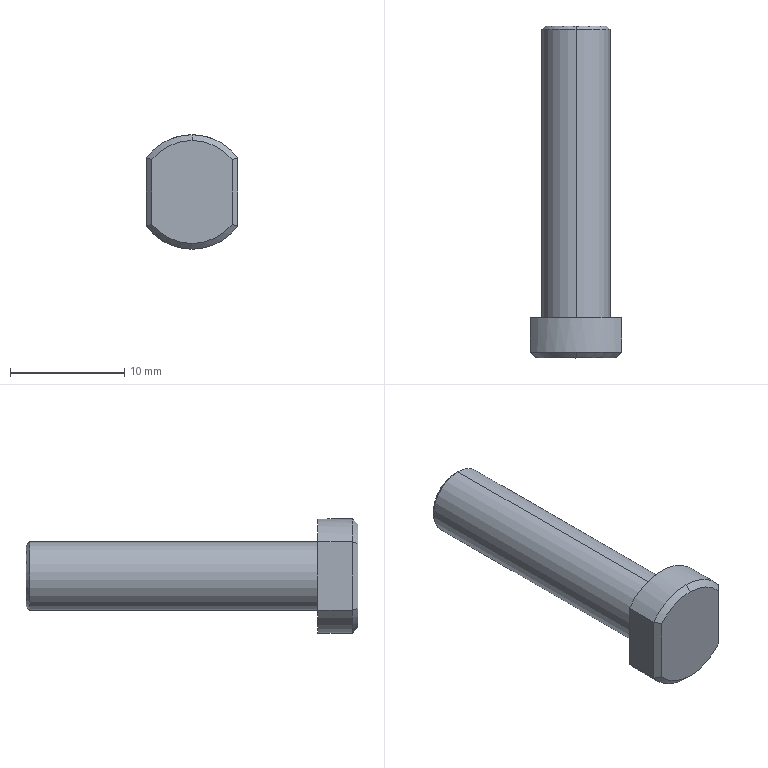Part | SolidWorks | features BaseBody 1 | 1 solid | 21 faces | box 8 x 29 x 10 mm | volume 861.581 mm3 | cone 7 | cylinder 7 | plane 7 | commonest cylinder face diameters 10 x3 3.3 x2 6 x2
STEP:
#1=CARTESIAN_POINT('',(0.,29.,2.7));
#2=VERTEX_POINT('',#1);
#3=CARTESIAN_POINT('',(0.,28.7,3.));
#4=VERTEX_POINT('',#3);
#5=CARTESIAN_POINT('',(0.,29.,2.7));
#6=DIRECTION('',(0.,-0.7071,0.7071));
#7=VECTOR('',#6,1000.);
#8=LINE('',#5,#7);
#9=EDGE_CURVE('',#2,#4,#8,.T.);
#10=ORIENTED_EDGE('',*,*,#9,.F.);
#11=CARTESIAN_POINT('',(0.,29.,-2.7));
#12=VERTEX_POINT('',#11);
#13=CARTESIAN_POINT('',(0.,29.,0.));
#14=DIRECTION('',(0.,1.,0.));
#15=DIRECTION('',(0.,0.,1.));
#16=AXIS2_PLACEMENT_3D('',#13,#14,#15);
#17=CIRCLE('',#16,2.7);
#18=EDGE_CURVE('',#12,#2,#17,.T.);
#19=ORIENTED_EDGE('',*,*,#18,.F.);
#20=CARTESIAN_POINT('',(0.,28.7,-3.));
#21=VERTEX_POINT('',#20);
#22=CARTESIAN_POINT('',(0.,29.,-2.7));
#23=DIRECTION('',(0.,-0.7071,-0.7071));
#24=VECTOR('',#23,1000.);
#25=LINE('',#22,#24);
#26=EDGE_CURVE('',#12,#21,#25,.T.);
#27=ORIENTED_EDGE('',*,*,#26,.T.);
#28=CARTESIAN_POINT('',(0.,28.7,0.));
#29=DIRECTION('',(0.,-1.,0.));
#30=DIRECTION('',(0.,0.,1.));
#31=AXIS2_PLACEMENT_3D('',#28,#29,#30);
#32=CIRCLE('',#31,3.);
#33=EDGE_CURVE('',#4,#21,#32,.T.);
#34=ORIENTED_EDGE('',*,*,#33,.F.);
#35=EDGE_LOOP('',(#10,#19,#27,#34));
#36=FACE_OUTER_BOUND('',#35,.T.);
#37=CARTESIAN_POINT('',(0.,29.,0.));
#38=DIRECTION('',(0.,-1.,0.));
#39=DIRECTION('',(0.,0.,-1.));
#40=AXIS2_PLACEMENT_3D('',#37,#38,#39);
#41=CONICAL_SURFACE('',#40,2.7,0.7854);
#42=ADVANCED_FACE('',(#36),#41,.T.);
#43=CARTESIAN_POINT('',(0.,17.5,-1.65));
#44=VERTEX_POINT('',#43);
#45=CARTESIAN_POINT('',(0.,29.,-1.65));
#46=VERTEX_POINT('',#45);
#47=CARTESIAN_POINT('',(0.,29.,-1.65));
#48=DIRECTION('',(0.,1.,0.));
#49=VECTOR('',#48,1000.);
#50=LINE('',#47,#49);
#51=EDGE_CURVE('',#44,#46,#50,.T.);
#52=ORIENTED_EDGE('',*,*,#51,.F.);
#53=CARTESIAN_POINT('',(0.,17.5,1.65));
#54=VERTEX_POINT('',#53);
#55=CARTESIAN_POINT('',(0.,17.5,0.));
#56=DIRECTION('',(0.,1.,0.));
#57=DIRECTION('',(0.,0.,1.));
#58=AXIS2_PLACEMENT_3D('',#55,#56,#57);
#59=CIRCLE('',#58,1.65);
#60=EDGE_CURVE('',#54,#44,#59,.T.);
#61=ORIENTED_EDGE('',*,*,#60,.F.);
#62=CARTESIAN_POINT('',(0.,29.,1.65));
#63=VERTEX_POINT('',#62);
#64=CARTESIAN_POINT('',(0.,29.,1.65));
#65=DIRECTION('',(0.,1.,0.));
#66=VECTOR('',#65,1000.);
#67=LINE('',#64,#66);
#68=EDGE_CURVE('',#54,#63,#67,.T.);
#69=ORIENTED_EDGE('',*,*,#68,.T.);
#70=CARTESIAN_POINT('',(0.,29.,0.));
#71=DIRECTION('',(0.,1.,0.));
#72=DIRECTION('',(0.,0.,1.));
#73=AXIS2_PLACEMENT_3D('',#70,#71,#72);
#74=CIRCLE('',#73,1.65);
#75=EDGE_CURVE('',#63,#46,#74,.T.);
#76=ORIENTED_EDGE('',*,*,#75,.T.);
#77=EDGE_LOOP('',(#52,#61,#69,#76));
#78=FACE_OUTER_BOUND('',#77,.T.);
#79=CARTESIAN_POINT('',(0.,29.,0.));
#80=DIRECTION('',(0.,1.,0.));
#81=DIRECTION('',(0.,0.,1.));
#82=AXIS2_PLACEMENT_3D('',#79,#80,#81);
#83=CYLINDRICAL_SURFACE('',#82,1.65);
#84=ADVANCED_FACE('',(#78),#83,.F.);
#85=CARTESIAN_POINT('',(0.,16.509,0.));
#86=VERTEX_POINT('',#85);
#87=CARTESIAN_POINT('',(0.,17.5,-1.65));
#88=DIRECTION('',(0.,0.515,-0.8572));
#89=VECTOR('',#88,1000.);
#90=LINE('',#87,#89);
#91=EDGE_CURVE('',#86,#44,#90,.T.);
#92=ORIENTED_EDGE('',*,*,#91,.F.);
#93=CARTESIAN_POINT('',(0.,17.5,1.65));
#94=DIRECTION('',(0.,0.515,0.8572));
#95=VECTOR('',#94,1000.);
#96=LINE('',#93,#95);
#97=EDGE_CURVE('',#86,#54,#96,.T.);
#98=ORIENTED_EDGE('',*,*,#97,.T.);
#99=ORIENTED_EDGE('',*,*,#60,.T.);
#100=EDGE_LOOP('',(#92,#98,#99));
#101=FACE_OUTER_BOUND('',#100,.T.);
#102=CARTESIAN_POINT('',(0.,17.5,0.));
#103=DIRECTION('',(0.,1.,0.));
#104=DIRECTION('',(0.,0.,1.));
#105=AXIS2_PLACEMENT_3D('',#102,#103,#104);
#106=CONICAL_SURFACE('',#105,1.65,1.03);
#107=ADVANCED_FACE('',(#101),#106,.F.);
#108=CARTESIAN_POINT('',(4.,0.5,3.));
#109=VERTEX_POINT('',#108);
#110=CARTESIAN_POINT('',(3.5,0.,2.828));
#111=VERTEX_POINT('',#110);
#112=CARTESIAN_POINT('',(4.,0.5,3.));
#113=CARTESIAN_POINT('',(3.833,0.3331,2.944));
#114=CARTESIAN_POINT('',(3.666,0.1664,2.887));
#115=CARTESIAN_POINT('',(3.5,0.,2.828));
#116=B_SPLINE_CURVE_WITH_KNOTS('',3,(#112,#113,#114,#115),.UNSPECIFIED.,.F.,.F.,(4,4),(0.,0.0007276),.UNSPECIFIED.);
#117=EDGE_CURVE('',#109,#111,#116,.T.);
#118=ORIENTED_EDGE('',*,*,#117,.T.);
#119=CARTESIAN_POINT('',(3.5,0.,-2.828));
#120=VERTEX_POINT('',#119);
#121=CARTESIAN_POINT('',(3.5,0.,0.));
#122=DIRECTION('',(0.,0.,1.));
#123=VECTOR('',#122,1000.);
#124=LINE('',#121,#123);
#125=EDGE_CURVE('',#120,#111,#124,.T.);
#126=ORIENTED_EDGE('',*,*,#125,.F.);
#127=CARTESIAN_POINT('',(4.,0.5,-3.));
#128=VERTEX_POINT('',#127);
#129=CARTESIAN_POINT('',(3.5,0.,-2.828));
#130=CARTESIAN_POINT('',(3.666,0.1664,-2.887));
#131=CARTESIAN_POINT('',(3.833,0.3331,-2.944));
#132=CARTESIAN_POINT('',(4.,0.5,-3.));
#133=B_SPLINE_CURVE_WITH_KNOTS('',3,(#129,#130,#131,#132),.UNSPECIFIED.,.F.,.F.,(4,4),(0.,0.0007276),.UNSPECIFIED.);
#134=EDGE_CURVE('',#120,#128,#133,.T.);
#135=ORIENTED_EDGE('',*,*,#134,.T.);
#136=CARTESIAN_POINT('',(4.,0.5,3.));
#137=DIRECTION('',(0.,0.,-1.));
#138=VECTOR('',#137,1000.);
#139=LINE('',#136,#138);
#140=EDGE_CURVE('',#109,#128,#139,.T.);
#141=ORIENTED_EDGE('',*,*,#140,.F.);
#142=EDGE_LOOP('',(#118,#126,#135,#141));
#143=FACE_OUTER_BOUND('',#142,.T.);
#144=CARTESIAN_POINT('',(4.,0.5,3.));
#145=DIRECTION('',(-0.7071,0.7071,0.));
#146=DIRECTION('',(0.,0.,1.));
#147=AXIS2_PLACEMENT_3D('',#144,#145,#146);
#148=PLANE('',#147);
#149=ADVANCED_FACE('',(#143),#148,.F.);
#150=CARTESIAN_POINT('',(-3.5,0.,-2.828));
#151=VERTEX_POINT('',#150);
#152=CARTESIAN_POINT('',(-4.,0.5,-3.));
#153=VERTEX_POINT('',#152);
#154=CARTESIAN_POINT('',(-3.5,0.,-2.828));
#155=CARTESIAN_POINT('',(-3.666,0.1664,-2.887));
#156=CARTESIAN_POINT('',(-3.833,0.3331,-2.944));
#157=CARTESIAN_POINT('',(-4.,0.5,-3.));
#158=B_SPLINE_CURVE_WITH_KNOTS('',3,(#154,#155,#156,#157),.UNSPECIFIED.,.F.,.F.,(4,4),(0.,0.0007276),.UNSPECIFIED.);
#159=EDGE_CURVE('',#151,#153,#158,.T.);
#160=ORIENTED_EDGE('',*,*,#159,.T.);
#161=CARTESIAN_POINT('',(0.,0.5,-5.));
#162=VERTEX_POINT('',#161);
#163=CARTESIAN_POINT('',(0.,0.5,0.));
#164=DIRECTION('',(0.,1.,0.));
#165=DIRECTION('',(0.,0.,1.));
#166=AXIS2_PLACEMENT_3D('',#163,#164,#165);
#167=CIRCLE('',#166,5.);
#168=EDGE_CURVE('',#162,#153,#167,.T.);
#169=ORIENTED_EDGE('',*,*,#168,.F.);
#170=CARTESIAN_POINT('',(0.,0.5,0.));
#171=DIRECTION('',(0.,1.,0.));
#172=DIRECTION('',(0.,0.,1.));
#173=AXIS2_PLACEMENT_3D('',#170,#171,#172);
#174=CIRCLE('',#173,5.);
#175=EDGE_CURVE('',#128,#162,#174,.T.);
#176=ORIENTED_EDGE('',*,*,#175,.F.);
#177=ORIENTED_EDGE('',*,*,#134,.F.);
#178=CARTESIAN_POINT('',(0.,0.,0.));
#179=DIRECTION('',(0.,-1.,0.));
#180=DIRECTION('',(0.,0.,1.));
#181=AXIS2_PLACEMENT_3D('',#178,#179,#180);
#182=CIRCLE('',#181,4.5);
#183=EDGE_CURVE('',#151,#120,#182,.T.);
#184=ORIENTED_EDGE('',*,*,#183,.F.);
#185=EDGE_LOOP('',(#160,#169,#176,#177,#184));
#186=FACE_OUTER_BOUND('',#185,.T.);
#187=CARTESIAN_POINT('',(0.,0.5,0.));
#188=DIRECTION('',(0.,1.,0.));
#189=DIRECTION('',(0.,0.,1.));
#190=AXIS2_PLACEMENT_3D('',#187,#188,#189);
#191=CONICAL_SURFACE('',#190,5.,0.7854);
#192=ADVANCED_FACE('',(#186),#191,.T.);
#193=CARTESIAN_POINT('',(0.,0.,4.5));
#194=VERTEX_POINT('',#193);
#195=CARTESIAN_POINT('',(0.,0.5,5.));
#196=VERTEX_POINT('',#195);
#197=CARTESIAN_POINT('',(0.,0.5,5.));
#198=DIRECTION('',(0.,0.7071,0.7071));
#199=VECTOR('',#198,1000.);
#200=LINE('',#197,#199);
#201=EDGE_CURVE('',#194,#196,#200,.T.);
#202=ORIENTED_EDGE('',*,*,#201,.F.);
#203=CARTESIAN_POINT('',(0.,0.,0.));
#204=DIRECTION('',(0.,-1.,0.));
#205=DIRECTION('',(0.,0.,1.));
#206=AXIS2_PLACEMENT_3D('',#203,#204,#205);
#207=CIRCLE('',#206,4.5);
#208=EDGE_CURVE('',#111,#194,#207,.T.);
#209=ORIENTED_EDGE('',*,*,#208,.F.);
#210=ORIENTED_EDGE('',*,*,#117,.F.);
#211=CARTESIAN_POINT('',(0.,0.5,0.));
#212=DIRECTION('',(0.,1.,0.));
#213=DIRECTION('',(0.,0.,1.));
#214=AXIS2_PLACEMENT_3D('',#211,#212,#213);
#215=CIRCLE('',#214,5.);
#216=EDGE_CURVE('',#196,#109,#215,.T.);
#217=ORIENTED_EDGE('',*,*,#216,.F.);
#218=EDGE_LOOP('',(#202,#209,#210,#217));
#219=FACE_OUTER_BOUND('',#218,.T.);
#220=CARTESIAN_POINT('',(0.,0.5,0.));
#221=DIRECTION('',(0.,1.,0.));
#222=DIRECTION('',(0.,0.,1.));
#223=AXIS2_PLACEMENT_3D('',#220,#221,#222);
#224=CONICAL_SURFACE('',#223,5.,0.7854);
#225=ADVANCED_FACE('',(#219),#224,.T.);
#226=ORIENTED_EDGE('',*,*,#159,.F.);
#227=CARTESIAN_POINT('',(-3.5,0.,2.828));
#228=VERTEX_POINT('',#227);
#229=CARTESIAN_POINT('',(-3.5,0.,0.));
#230=DIRECTION('',(0.,0.,-1.));
#231=VECTOR('',#230,1000.);
#232=LINE('',#229,#231);
#233=EDGE_CURVE('',#228,#151,#232,.T.);
#234=ORIENTED_EDGE('',*,*,#233,.F.);
#235=CARTESIAN_POINT('',(-4.,0.5,3.));
#236=VERTEX_POINT('',#235);
#237=CARTESIAN_POINT('',(-4.,0.5,3.));
#238=CARTESIAN_POINT('',(-3.833,0.3331,2.944));
#239=CARTESIAN_POINT('',(-3.666,0.1664,2.887));
#240=CARTESIAN_POINT('',(-3.5,0.,2.828));
#241=B_SPLINE_CURVE_WITH_KNOTS('',3,(#237,#238,#239,#240),.UNSPECIFIED.,.F.,.F.,(4,4),(0.,0.0007276),.UNSPECIFIED.);
#242=EDGE_CURVE('',#236,#228,#241,.T.);
#243=ORIENTED_EDGE('',*,*,#242,.F.);
#244=CARTESIAN_POINT('',(-4.,0.5,3.));
#245=DIRECTION('',(0.,0.,1.));
#246=VECTOR('',#245,1000.);
#247=LINE('',#244,#246);
#248=EDGE_CURVE('',#153,#236,#247,.T.);
#249=ORIENTED_EDGE('',*,*,#248,.F.);
#250=EDGE_LOOP('',(#226,#234,#243,#249));
#251=FACE_OUTER_BOUND('',#250,.T.);
#252=CARTESIAN_POINT('',(-4.,0.5,3.));
#253=DIRECTION('',(0.7071,0.7071,0.));
#254=DIRECTION('',(0.,0.,-1.));
#255=AXIS2_PLACEMENT_3D('',#252,#253,#254);
#256=PLANE('',#255);
#257=ADVANCED_FACE('',(#251),#256,.F.);
#258=CARTESIAN_POINT('',(-4.,3.5,-3.));
#259=VERTEX_POINT('',#258);
#260=CARTESIAN_POINT('',(-4.,29.001,-3.));
#261=DIRECTION('',(0.,-1.,0.));
#262=VECTOR('',#261,1000.);
#263=LINE('',#260,#262);
#264=EDGE_CURVE('',#259,#153,#263,.T.);
#265=ORIENTED_EDGE('',*,*,#264,.T.);
#266=ORIENTED_EDGE('',*,*,#248,.T.);
#267=CARTESIAN_POINT('',(-4.,3.5,3.));
#268=VERTEX_POINT('',#267);
#269=CARTESIAN_POINT('',(-4.,29.001,3.));
#270=DIRECTION('',(0.,-1.,0.));
#271=VECTOR('',#270,1000.);
#272=LINE('',#269,#271);
#273=EDGE_CURVE('',#268,#236,#272,.T.);
#274=ORIENTED_EDGE('',*,*,#273,.F.);
#275=CARTESIAN_POINT('',(-4.,3.5,3.));
#276=DIRECTION('',(0.,0.,1.));
#277=VECTOR('',#276,1000.);
#278=LINE('',#275,#277);
#279=EDGE_CURVE('',#259,#268,#278,.T.);
#280=ORIENTED_EDGE('',*,*,#279,.F.);
#281=EDGE_LOOP('',(#265,#266,#274,#280));
#282=FACE_OUTER_BOUND('',#281,.T.);
#283=CARTESIAN_POINT('',(-4.,29.001,3.));
#284=DIRECTION('',(1.,0.,0.));
#285=DIRECTION('',(0.,1.,0.));
#286=AXIS2_PLACEMENT_3D('',#283,#284,#285);
#287=PLANE('',#286);
#288=ADVANCED_FACE('',(#282),#287,.F.);
#289=CARTESIAN_POINT('',(4.,3.5,3.));
#290=VERTEX_POINT('',#289);
#291=CARTESIAN_POINT('',(4.,29.001,3.));
#292=DIRECTION('',(0.,-1.,0.));
#293=VECTOR('',#292,1000.);
#294=LINE('',#291,#293);
#295=EDGE_CURVE('',#290,#109,#294,.T.);
#296=ORIENTED_EDGE('',*,*,#295,.T.);
#297=ORIENTED_EDGE('',*,*,#140,.T.);
#298=CARTESIAN_POINT('',(4.,3.5,-3.));
#299=VERTEX_POINT('',#298);
#300=CARTESIAN_POINT('',(4.,29.001,-3.));
#301=DIRECTION('',(0.,-1.,0.));
#302=VECTOR('',#301,1000.);
#303=LINE('',#300,#302);
#304=EDGE_CURVE('',#299,#128,#303,.T.);
#305=ORIENTED_EDGE('',*,*,#304,.F.);
#306=CARTESIAN_POINT('',(4.,3.5,3.));
#307=DIRECTION('',(0.,0.,-1.));
#308=VECTOR('',#307,1000.);
#309=LINE('',#306,#308);
#310=EDGE_CURVE('',#290,#299,#309,.T.);
#311=ORIENTED_EDGE('',*,*,#310,.F.);
#312=EDGE_LOOP('',(#296,#297,#305,#311));
#313=FACE_OUTER_BOUND('',#312,.T.);
#314=CARTESIAN_POINT('',(4.,29.001,3.));
#315=DIRECTION('',(-1.,0.,0.));
#316=DIRECTION('',(0.,0.,1.));
#317=AXIS2_PLACEMENT_3D('',#314,#315,#316);
#318=PLANE('',#317);
#319=ADVANCED_FACE('',(#313),#318,.F.);
#320=ORIENTED_EDGE('',*,*,#75,.F.);
#321=CARTESIAN_POINT('',(0.,29.,0.));
#322=DIRECTION('',(0.,1.,0.));
#323=DIRECTION('',(0.,0.,1.));
#324=AXIS2_PLACEMENT_3D('',#321,#322,#323);
#325=CIRCLE('',#324,1.65);
#326=EDGE_CURVE('',#46,#63,#325,.T.);
#327=ORIENTED_EDGE('',*,*,#326,.F.);
#328=EDGE_LOOP('',(#320,#327));
#329=FACE_BOUND('',#328,.T.);
#330=ORIENTED_EDGE('',*,*,#18,.T.);
#331=CARTESIAN_POINT('',(0.,29.,0.));
#332=DIRECTION('',(0.,1.,0.));
#333=DIRECTION('',(0.,0.,1.));
#334=AXIS2_PLACEMENT_3D('',#331,#332,#333);
#335=CIRCLE('',#334,2.7);
#336=EDGE_CURVE('',#2,#12,#335,.T.);
#337=ORIENTED_EDGE('',*,*,#336,.T.);
#338=EDGE_LOOP('',(#330,#337));
#339=FACE_OUTER_BOUND('',#338,.T.);
#340=CARTESIAN_POINT('',(0.,29.,0.));
#341=DIRECTION('',(0.,1.,0.));
#342=DIRECTION('',(1.,0.,0.));
#343=AXIS2_PLACEMENT_3D('',#340,#341,#342);
#344=PLANE('',#343);
#345=ADVANCED_FACE('',(#329,#339),#344,.T.);
#346=CARTESIAN_POINT('',(0.,3.5,-3.));
#347=VERTEX_POINT('',#346);
#348=CARTESIAN_POINT('',(0.,3.5,-3.));
#349=DIRECTION('',(0.,1.,0.));
#350=VECTOR('',#349,1000.);
#351=LINE('',#348,#350);
#352=EDGE_CURVE('',#347,#21,#351,.T.);
#353=ORIENTED_EDGE('',*,*,#352,.F.);
#354=CARTESIAN_POINT('',(0.,3.5,3.));
#355=VERTEX_POINT('',#354);
#356=CARTESIAN_POINT('',(0.,3.5,0.));
#357=DIRECTION('',(0.,1.,0.));
#358=DIRECTION('',(0.,0.,1.));
#359=AXIS2_PLACEMENT_3D('',#356,#357,#358);
#360=CIRCLE('',#359,3.);
#361=EDGE_CURVE('',#347,#355,#360,.T.);
#362=ORIENTED_EDGE('',*,*,#361,.T.);
#363=CARTESIAN_POINT('',(0.,3.5,3.));
#364=DIRECTION('',(0.,1.,0.));
#365=VECTOR('',#364,1000.);
#366=LINE('',#363,#365);
#367=EDGE_CURVE('',#355,#4,#366,.T.);
#368=ORIENTED_EDGE('',*,*,#367,.T.);
#369=ORIENTED_EDGE('',*,*,#33,.T.);
#370=EDGE_LOOP('',(#353,#362,#368,#369));
#371=FACE_OUTER_BOUND('',#370,.T.);
#372=CARTESIAN_POINT('',(0.,3.5,0.));
#373=DIRECTION('',(0.,1.,0.));
#374=DIRECTION('',(0.,0.,1.));
#375=AXIS2_PLACEMENT_3D('',#372,#373,#374);
#376=CYLINDRICAL_SURFACE('',#375,3.);
#377=ADVANCED_FACE('',(#371),#376,.T.);
#378=CARTESIAN_POINT('',(0.,3.5,0.));
#379=DIRECTION('',(0.,1.,0.));
#380=DIRECTION('',(0.,0.,1.));
#381=AXIS2_PLACEMENT_3D('',#378,#379,#380);
#382=CIRCLE('',#381,3.);
#383=EDGE_CURVE('',#355,#347,#382,.T.);
#384=ORIENTED_EDGE('',*,*,#383,.F.);
#385=ORIENTED_EDGE('',*,*,#361,.F.);
#386=EDGE_LOOP('',(#384,#385));
#387=FACE_BOUND('',#386,.T.);
#388=ORIENTED_EDGE('',*,*,#279,.T.);
#389=CARTESIAN_POINT('',(0.,3.5,0.));
#390=DIRECTION('',(0.,1.,0.));
#391=DIRECTION('',(0.,0.,1.));
#392=AXIS2_PLACEMENT_3D('',#389,#390,#391);
#393=CIRCLE('',#392,5.);
#394=EDGE_CURVE('',#268,#290,#393,.T.);
#395=ORIENTED_EDGE('',*,*,#394,.T.);
#396=ORIENTED_EDGE('',*,*,#310,.T.);
#397=CARTESIAN_POINT('',(0.,3.5,-5.));
#398=VERTEX_POINT('',#397);
#399=CARTESIAN_POINT('',(0.,3.5,0.));
#400=DIRECTION('',(0.,1.,0.));
#401=DIRECTION('',(0.,0.,1.));
#402=AXIS2_PLACEMENT_3D('',#399,#400,#401);
#403=CIRCLE('',#402,5.);
#404=EDGE_CURVE('',#299,#398,#403,.T.);
#405=ORIENTED_EDGE('',*,*,#404,.T.);
#406=CARTESIAN_POINT('',(0.,3.5,0.));
#407=DIRECTION('',(0.,1.,0.));
#408=DIRECTION('',(0.,0.,1.));
#409=AXIS2_PLACEMENT_3D('',#406,#407,#408);
#410=CIRCLE('',#409,5.);
#411=EDGE_CURVE('',#398,#259,#410,.T.);
#412=ORIENTED_EDGE('',*,*,#411,.T.);
#413=EDGE_LOOP('',(#388,#395,#396,#405,#412));
#414=FACE_OUTER_BOUND('',#413,.T.);
#415=CARTESIAN_POINT('',(0.,3.5,0.));
#416=DIRECTION('',(0.,1.,0.));
#417=DIRECTION('',(1.,0.,0.));
#418=AXIS2_PLACEMENT_3D('',#415,#416,#417);
#419=PLANE('',#418);
#420=ADVANCED_FACE('',(#387,#414),#419,.T.);
#421=ORIENTED_EDGE('',*,*,#183,.T.);
#422=ORIENTED_EDGE('',*,*,#125,.T.);
#423=ORIENTED_EDGE('',*,*,#208,.T.);
#424=CARTESIAN_POINT('',(0.,0.,0.));
#425=DIRECTION('',(0.,-1.,0.));
#426=DIRECTION('',(0.,0.,1.));
#427=AXIS2_PLACEMENT_3D('',#424,#425,#426);
#428=CIRCLE('',#427,4.5);
#429=EDGE_CURVE('',#194,#228,#428,.T.);
#430=ORIENTED_EDGE('',*,*,#429,.T.);
#431=ORIENTED_EDGE('',*,*,#233,.T.);
#432=EDGE_LOOP('',(#421,#422,#423,#430,#431));
#433=FACE_OUTER_BOUND('',#432,.T.);
#434=CARTESIAN_POINT('',(0.,0.,0.));
#435=DIRECTION('',(0.,1.,0.));
#436=DIRECTION('',(1.,0.,0.));
#437=AXIS2_PLACEMENT_3D('',#434,#435,#436);
#438=PLANE('',#437);
#439=ADVANCED_FACE('',(#433),#438,.F.);
#440=CARTESIAN_POINT('',(0.,29.,-5.));
#441=DIRECTION('',(0.,-1.,0.));
#442=VECTOR('',#441,1000.);
#443=LINE('',#440,#442);
#444=EDGE_CURVE('',#398,#162,#443,.T.);
#445=ORIENTED_EDGE('',*,*,#444,.F.);
#446=ORIENTED_EDGE('',*,*,#404,.F.);
#447=ORIENTED_EDGE('',*,*,#304,.T.);
#448=ORIENTED_EDGE('',*,*,#175,.T.);
#449=EDGE_LOOP('',(#445,#446,#447,#448));
#450=FACE_OUTER_BOUND('',#449,.T.);
#451=CARTESIAN_POINT('',(0.,29.,0.));
#452=DIRECTION('',(0.,-1.,0.));
#453=DIRECTION('',(0.,0.,-1.));
#454=AXIS2_PLACEMENT_3D('',#451,#452,#453);
#455=CYLINDRICAL_SURFACE('',#454,5.);
#456=ADVANCED_FACE('',(#450),#455,.T.);
#457=ORIENTED_EDGE('',*,*,#273,.T.);
#458=CARTESIAN_POINT('',(0.,0.5,0.));
#459=DIRECTION('',(0.,1.,0.));
#460=DIRECTION('',(0.,0.,1.));
#461=AXIS2_PLACEMENT_3D('',#458,#459,#460);
#462=CIRCLE('',#461,5.);
#463=EDGE_CURVE('',#236,#196,#462,.T.);
#464=ORIENTED_EDGE('',*,*,#463,.T.);
#465=ORIENTED_EDGE('',*,*,#216,.T.);
#466=ORIENTED_EDGE('',*,*,#295,.F.);
#467=ORIENTED_EDGE('',*,*,#394,.F.);
#468=EDGE_LOOP('',(#457,#464,#465,#466,#467));
#469=FACE_OUTER_BOUND('',#468,.T.);
#470=CARTESIAN_POINT('',(0.,29.,0.));
#471=DIRECTION('',(0.,-1.,0.));
#472=DIRECTION('',(0.,0.,-1.));
#473=AXIS2_PLACEMENT_3D('',#470,#471,#472);
#474=CYLINDRICAL_SURFACE('',#473,5.);
#475=ADVANCED_FACE('',(#469),#474,.T.);
#476=ORIENTED_EDGE('',*,*,#411,.F.);
#477=ORIENTED_EDGE('',*,*,#444,.T.);
#478=ORIENTED_EDGE('',*,*,#168,.T.);
#479=ORIENTED_EDGE('',*,*,#264,.F.);
#480=EDGE_LOOP('',(#476,#477,#478,#479));
#481=FACE_OUTER_BOUND('',#480,.T.);
#482=CARTESIAN_POINT('',(0.,29.,0.));
#483=DIRECTION('',(0.,-1.,0.));
#484=DIRECTION('',(0.,0.,-1.));
#485=AXIS2_PLACEMENT_3D('',#482,#483,#484);
#486=CYLINDRICAL_SURFACE('',#485,5.);
#487=ADVANCED_FACE('',(#481),#486,.T.);
#488=ORIENTED_EDGE('',*,*,#383,.T.);
#489=ORIENTED_EDGE('',*,*,#352,.T.);
#490=CARTESIAN_POINT('',(0.,28.7,0.));
#491=DIRECTION('',(0.,-1.,0.));
#492=DIRECTION('',(0.,0.,1.));
#493=AXIS2_PLACEMENT_3D('',#490,#491,#492);
#494=CIRCLE('',#493,3.);
#495=EDGE_CURVE('',#21,#4,#494,.T.);
#496=ORIENTED_EDGE('',*,*,#495,.T.);
#497=ORIENTED_EDGE('',*,*,#367,.F.);
#498=EDGE_LOOP('',(#488,#489,#496,#497));
#499=FACE_OUTER_BOUND('',#498,.T.);
#500=CARTESIAN_POINT('',(0.,3.5,0.));
#501=DIRECTION('',(0.,1.,0.));
#502=DIRECTION('',(0.,0.,1.));
#503=AXIS2_PLACEMENT_3D('',#500,#501,#502);
#504=CYLINDRICAL_SURFACE('',#503,3.);
#505=ADVANCED_FACE('',(#499),#504,.T.);
#506=ORIENTED_EDGE('',*,*,#429,.F.);
#507=ORIENTED_EDGE('',*,*,#201,.T.);
#508=ORIENTED_EDGE('',*,*,#463,.F.);
#509=ORIENTED_EDGE('',*,*,#242,.T.);
#510=EDGE_LOOP('',(#506,#507,#508,#509));
#511=FACE_OUTER_BOUND('',#510,.T.);
#512=CARTESIAN_POINT('',(0.,0.5,0.));
#513=DIRECTION('',(0.,1.,0.));
#514=DIRECTION('',(0.,0.,1.));
#515=AXIS2_PLACEMENT_3D('',#512,#513,#514);
#516=CONICAL_SURFACE('',#515,5.,0.7854);
#517=ADVANCED_FACE('',(#511),#516,.T.);
#518=ORIENTED_EDGE('',*,*,#97,.F.);
#519=ORIENTED_EDGE('',*,*,#91,.T.);
#520=CARTESIAN_POINT('',(0.,17.5,0.));
#521=DIRECTION('',(0.,1.,0.));
#522=DIRECTION('',(0.,0.,1.));
#523=AXIS2_PLACEMENT_3D('',#520,#521,#522);
#524=CIRCLE('',#523,1.65);
#525=EDGE_CURVE('',#44,#54,#524,.T.);
#526=ORIENTED_EDGE('',*,*,#525,.T.);
#527=EDGE_LOOP('',(#518,#519,#526));
#528=FACE_OUTER_BOUND('',#527,.T.);
#529=CARTESIAN_POINT('',(0.,17.5,0.));
#530=DIRECTION('',(0.,1.,0.));
#531=DIRECTION('',(0.,0.,1.));
#532=AXIS2_PLACEMENT_3D('',#529,#530,#531);
#533=CONICAL_SURFACE('',#532,1.65,1.03);
#534=ADVANCED_FACE('',(#528),#533,.F.);
#535=ORIENTED_EDGE('',*,*,#525,.F.);
#536=ORIENTED_EDGE('',*,*,#51,.T.);
#537=ORIENTED_EDGE('',*,*,#326,.T.);
#538=ORIENTED_EDGE('',*,*,#68,.F.);
#539=EDGE_LOOP('',(#535,#536,#537,#538));
#540=FACE_OUTER_BOUND('',#539,.T.);
#541=CARTESIAN_POINT('',(0.,29.,0.));
#542=DIRECTION('',(0.,1.,0.));
#543=DIRECTION('',(0.,0.,1.));
#544=AXIS2_PLACEMENT_3D('',#541,#542,#543);
#545=CYLINDRICAL_SURFACE('',#544,1.65);
#546=ADVANCED_FACE('',(#540),#545,.F.);
#547=ORIENTED_EDGE('',*,*,#336,.F.);
#548=ORIENTED_EDGE('',*,*,#9,.T.);
#549=ORIENTED_EDGE('',*,*,#495,.F.);
#550=ORIENTED_EDGE('',*,*,#26,.F.);
#551=EDGE_LOOP('',(#547,#548,#549,#550));
#552=FACE_OUTER_BOUND('',#551,.T.);
#553=CARTESIAN_POINT('',(0.,29.,0.));
#554=DIRECTION('',(0.,-1.,0.));
#555=DIRECTION('',(0.,0.,-1.));
#556=AXIS2_PLACEMENT_3D('',#553,#554,#555);
#557=CONICAL_SURFACE('',#556,2.7,0.7854);
#558=ADVANCED_FACE('',(#552),#557,.T.);
#559=CLOSED_SHELL('',(#42,#84,#107,#149,#192,#225,#257,#288,#319,#345,#377,#420,#439,#456,#475,#487,#505,#517,#534,#546,#558));
#560=MANIFOLD_SOLID_BREP('',#559);
#561=CARTESIAN_POINT('',(0.,0.,0.));
#562=DIRECTION('',(0.,0.,1.));
#563=DIRECTION('',(1.,0.,0.));
#564=AXIS2_PLACEMENT_3D('',#561,#562,#563);
#565=(LENGTH_UNIT()NAMED_UNIT(*)SI_UNIT(.MILLI.,.METRE.));
#566=UNCERTAINTY_MEASURE_WITH_UNIT(LENGTH_MEASURE(0.00001),#565,'','');
#567=(NAMED_UNIT(*)PLANE_ANGLE_UNIT()SI_UNIT($,.RADIAN.));
#568=(NAMED_UNIT(*)SI_UNIT($,.STERADIAN.)SOLID_ANGLE_UNIT());
#569=(GEOMETRIC_REPRESENTATION_CONTEXT(3)GLOBAL_UNCERTAINTY_ASSIGNED_CONTEXT((#566))GLOBAL_UNIT_ASSIGNED_CONTEXT((#565,#567,#568))REPRESENTATION_CONTEXT('',''));
#570=ADVANCED_BREP_SHAPE_REPRESENTATION('',(#560,#564),#569);